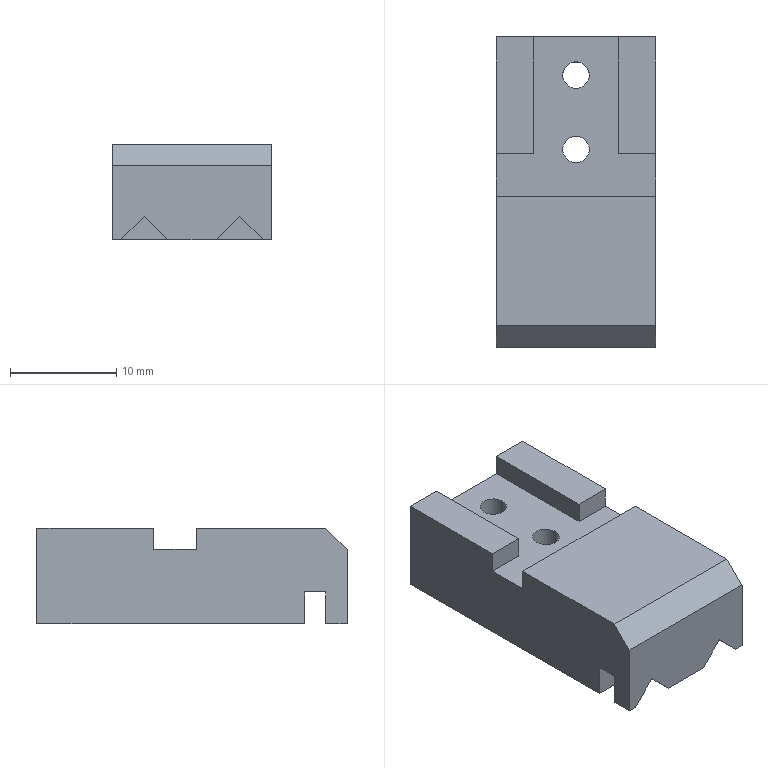Part | STEP file | A05-1 | 1 solid | 29 faces | box 15 x 29.2 x 9 mm | volume 3438 mm3 | plane 25 | cylinder 4 | commonest cylinder face diameters 2.5 x4